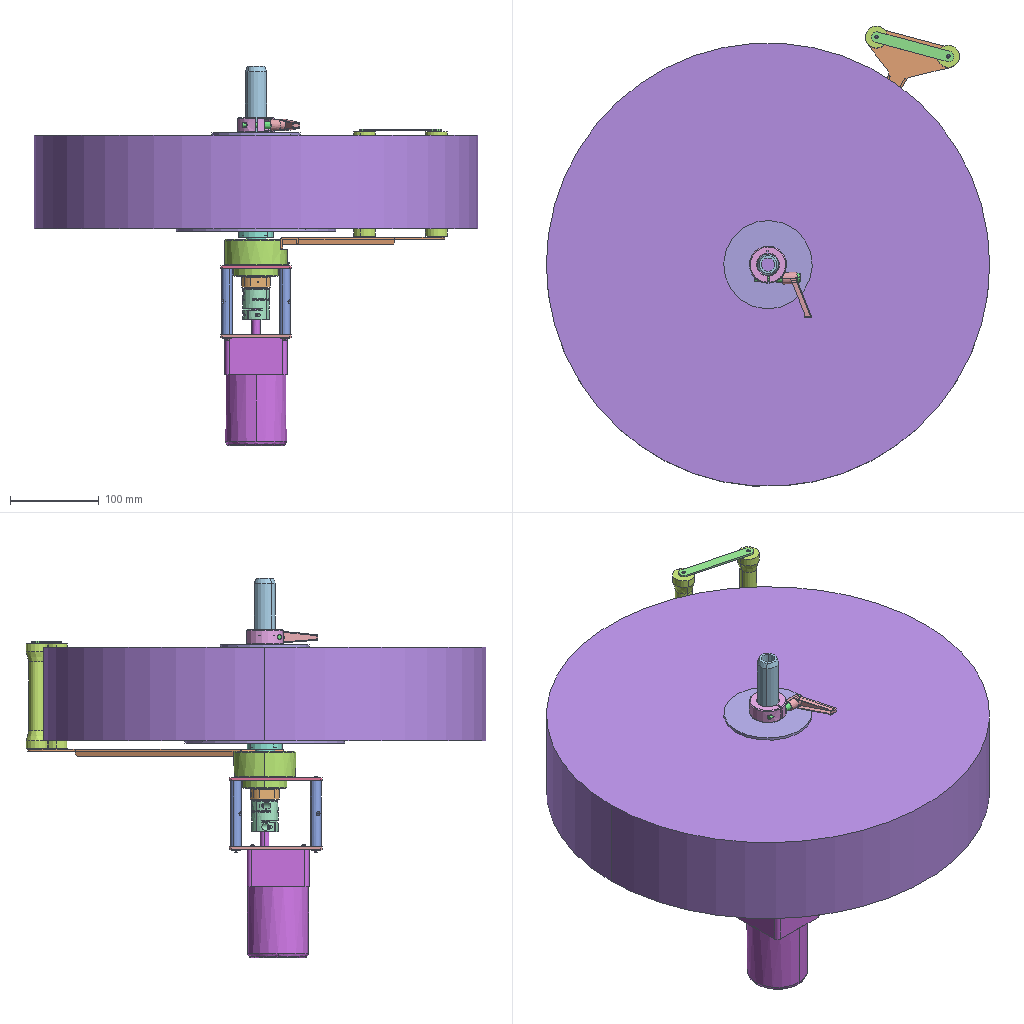Assembly | SolidWorks | 29 different items | 84 placed | box 500 x 519 x 428 mm
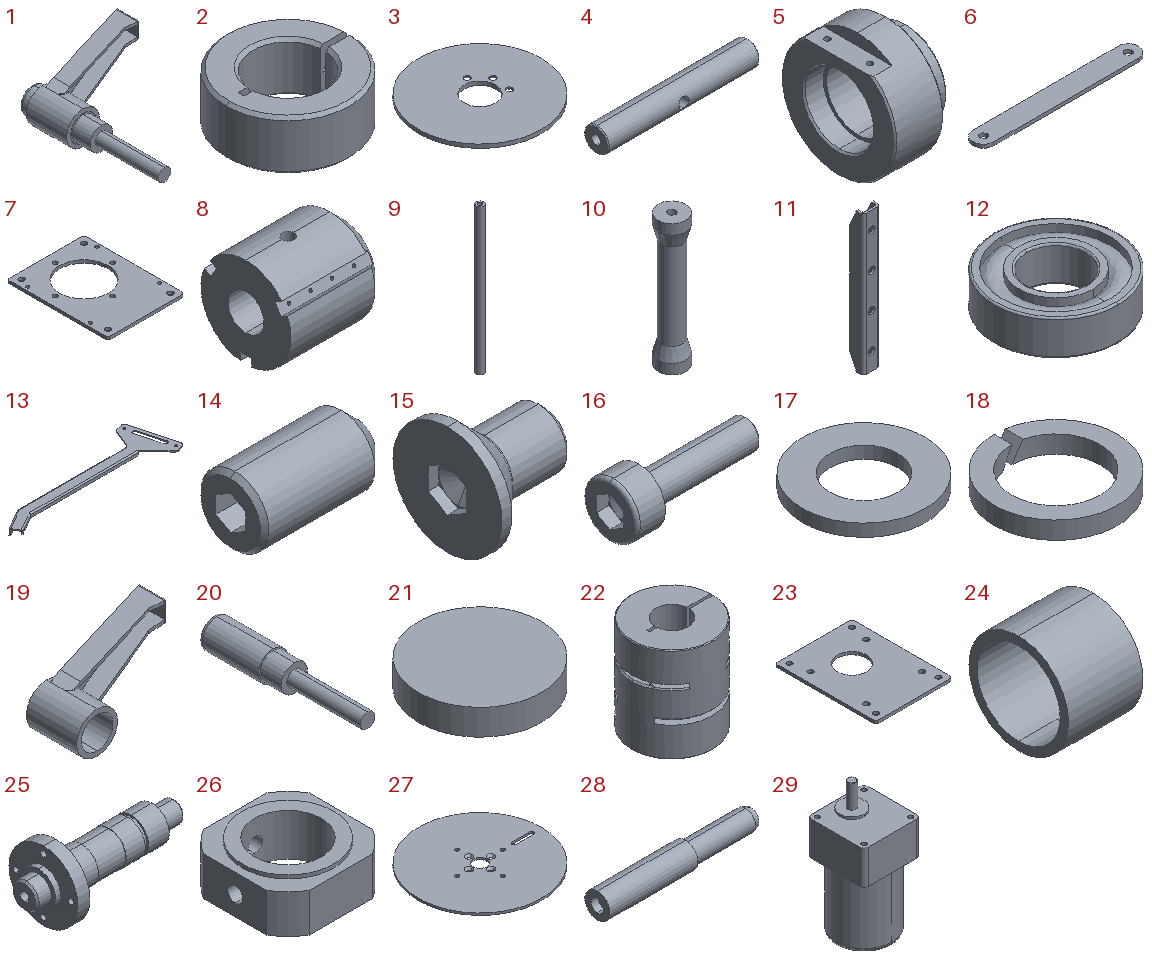Parts list (item | name | quantity | parent item | size | volume | features):
1 | (subassembly) | x1 | - | 51.5 x 63.5 x 13 mm | 4259 mm3 | -
2 | - | x1 | - | 41.976 x 42 x 17 mm | 13853 mm3 | features ICE 7, Chamfer 2, HoleWzd 2
3 | - | x1 | - | 100 x 100 x 3 mm | 21741 mm3 | features Extrusion 1, HoleWzd 1
4 | - | x4 | - | 75 x 12 x 12 mm | 7888 mm3 | features HoleWzd 2, Chamfer 1, Extrusion 1, ICE 1
5 | - | x1 | - | 42 x 70 x 70 mm | 81911 mm3 | features ICE 5, HoleWzd 2, Chamfer 1, CirPattern 1, Cut 1, Extrusion 1
6 | - | x1 | - | 96 x 12 x 2 mm | 2187 mm3 | features Extrusion 1, HoleWzd 1
7 | - | x1 | - | 80 x 105 x 3 mm | 18683 mm3 | features HoleWzd 2, Chamfer 1, Extrusion 1, ICE 1
8 | - | x1 | - | 80 x 75 x 74.698 mm | 269789 mm3 | features CirPattern 2, HoleWzd 2, ICE 2, Chamfer 1, Revolution 1
9 | - | x2 | - | 6 x 6 x 120 mm | 3214 mm3 | features HoleWzd 2, Extrusion 1
10 | - | x2 | - | 25 x 25 x 118 mm | 35489 mm3 | features Extrusion 1, RevCut 1
11 | - | x3 | - | 8.8 x 7 x 72 mm | 1341 mm3 | features Chamfer 2, FlatPattern 1, HoleWzd 1, SMBaseFlange 1, SheetMetal 1
12 | - | x2 | - | 42 x 42 x 12 mm | 10656 mm3 | features BaseBody 1
13 | - | x1 | - | 320.025 x 100.043 x 14 mm | 22575 mm3 | features ICE 5, Chamfer 2, HoleWzd 2, 3DProfileFeature 1, EdgeFlange 1, Fillet 1, FlatPattern 1, SMBaseFlange 1, SheetMetal 1
14 | - | x4 | - | 3 x 1.6 x 1.6 mm | 5.35 mm3 | features RevCut 2, Cut 1, LPattern 1, Revolution 1
15 | - | x4 | - | 10 x 11.34 x 11.34 mm | 423.495 mm3 | features RevCut 3, Chamfer 1, Cut 1, Fillet 1, LPattern 1, Revolution 1
16 | - | x20 | - | 7.6 x 3 x 3 mm | 21.652 mm3 | features Fillet 2, RevCut 2, Boss 1, Chamfer 1, Cut 1, Extrusion 1, LPattern 1
17 | - | x12 | - | 10 x 10 x 1 mm | 54.782 mm3 | features Extrusion 1
18 | - | x12 | - | 4.2 x 4.2 x 0.6 mm | 3.946 mm3 | features Cut 1, Extrusion 1
19 | - | x1 | in 1 | 51.5 x 31.3 x 13 mm | 1733 mm3 | features BaseBody 1, Shell 1
20 | - | x1 | in 1 | 10 x 52.5 x 10 mm | 2526 mm3 | features ICE 3, BaseBody 1
21 | - | x1 | - | 500 x 500 x 105 mm | 20616702 mm3 | features Extrusion 1
22 | - | x1 | - | 30 x 30 x 35 mm | 19054 mm3 | features BaseBody 1
23 | - | x1 | - | 80 x 105 x 3 mm | 22444 mm3 | features ICE 2, Chamfer 1, Extrusion 1, HoleWzd 1
24 | - | x1 | - | 18 x 24 x 24 mm | 2488 mm3 | features Extrusion 1
25 | - | x1 | - | 87 x 40 x 40 mm | 29288 mm3 | features HoleWzd 2, Chamfer 1, RevCut 1, Revolution 1
26 | - | x1 | - | 30 x 30 x 12 mm | 6216 mm3 | features HoleWzd 2, ICE 2, Extrusion 1
27 | - | x1 | - | 180 x 180 x 3 mm | 74053 mm3 | features Chamfer 1, Extrusion 1, ICE 1
28 | - | x1 | - | 183 x 30 x 30 mm | 80329 mm3 | features Chamfer 1, Revolution 1
29 | - | x1 | - | 70 x 70 x 154 mm | 503318 mm3 | features BaseBody 1
Mates (type | each side: item.copy, entity, surface, feature):
Coincident | 23.1 face plane Boss-Extrude1 | 4.1 face plane Boss-Extrude1
Concentric | 23.1 face cylinder Cut-Extrude1 | 4.1 face cylinder M5 Tapped Hole2
Coincident | 23.1 face plane Boss-Extrude1 | 4.2 face plane Boss-Extrude1
Concentric | 23.1 face cylinder Cut-Extrude1 | 4.2 face cylinder M5 Tapped Hole2
Coincident | 23.1 face plane Boss-Extrude1 | 4.3 face plane Boss-Extrude1
Concentric | 23.1 face cylinder Cut-Extrude1 | 4.3 face cylinder M5 Tapped Hole2
Coincident | 23.1 face plane Boss-Extrude1 | 4.4 face plane Boss-Extrude1
Concentric | 23.1 face cylinder Cut-Extrude1 | 4.4 face cylinder M5 Tapped Hole2
Coincident | 4.2 face plane Boss-Extrude1 | 7.1 face plane Boss-Extrude1
Concentric | 4.2 face cylinder M5 Tapped Hole1 | 7.1 face cylinder Cut-Extrude1
Concentric | 4.3 face cylinder M5 Tapped Hole1 | 7.1 face cylinder Cut-Extrude1
Concentric | 5.1 face cylinder Boss-Extrude1 | 7.1 face cylinder Cut-Extrude1
Concentric | 5.1 face cylinder Cut-Extrude1 | 25.1 face cylinder Revolve1
Concentric | 25.1 face cylinder Revolve1 | 27.1 face cylinder Boss-Extrude1
Concentric | 25.1 face cylinder M4 Tapped Hole1 | 27.1 face cylinder Cut-Extrude1
Coincident | 25.1 face plane Revolve1 | 27.1 face plane Boss-Extrude1
Concentric | 24.1 face cylinder Boss-Extrude1 | 25.1 face cylinder Revolve1
Coincident | 5.1 face plane Cut-Extrude3 | 24.1 face plane Boss-Extrude1
Concentric | 25.1 face cylinder Revolve1 | 26.1 face cylinder Cut-Extrude1
Coincident | 5.1 face plane Boss-Extrude3 | 26.1 face plane Boss-Extrude2
Concentric | 25.1 face cylinder Revolve1 | 28.1 face cylinder Revolve1
Coincident | 27.1 face plane Boss-Extrude1 | 28.1 face plane Revolve1
Concentric | 28.1 face cylinder Revolve1 | 8.1 face cylinder Revolve1
Coincident | 27.1 face plane Boss-Extrude1 | 8.1 face plane Revolve1
Concentric | 23.1 face cylinder Cut-Extrude1 | 29.1 face cylinder Import1
Coincident | 23.1 face plane Boss-Extrude1 | 29.1 face plane Import1
Concentric | 29.1 face cylinder Import1 | 23.1 face cylinder Cut-Extrude3
Concentric | 25.1 face cylinder Revolve1 | 22.1 face cylinder Import1
Concentric | 5.1 face cylinder Cut-Extrude3 | 12.1 face cylinder Import1
Coincident | 5.1 face plane Cut-Extrude3 | 12.1 face plane Import1
Concentric | 5.1 face cylinder Cut-Extrude1 | 12.2 face cylinder Import1
Coincident | 5.1 face plane Cut-Extrude1 | 12.2 face plane Import1
Concentric | 29.1 face cylinder Import1 | 17.1 face cylinder Base-Extrude
Coincident | 23.1 face plane Boss-Extrude1 | 17.1 face plane Base-Extrude
Concentric | 29.1 face cylinder Import1 | 17.2 face cylinder Base-Extrude
Coincident | 23.1 face plane Boss-Extrude1 | 17.2 face plane Base-Extrude
Concentric | 29.1 face cylinder Import1 | 17.3 face cylinder Base-Extrude
Coincident | 23.1 face plane Boss-Extrude1 | 17.3 face plane Base-Extrude
Concentric | 29.1 face cylinder Import1 | 17.4 face cylinder Base-Extrude
Coincident | 23.1 face plane Boss-Extrude1 | 17.4 face plane Base-Extrude
Concentric | 17.4 face cylinder Base-Extrude | 18.1 face cylinder Base-Extrude
Coincident | 17.4 face plane Base-Extrude | 18.1 face plane Base-Extrude
Concentric | 17.3 face cylinder Base-Extrude | 18.2 face cylinder Base-Extrude
Coincident | 17.3 face plane Base-Extrude | 18.2 face plane Base-Extrude
Concentric | 17.2 face cylinder Base-Extrude | 18.3 face cylinder Base-Extrude
Coincident | 17.2 face plane Base-Extrude | 18.3 face plane Base-Extrude
Concentric | 17.1 face cylinder Base-Extrude | 18.4 face cylinder Base-Extrude
Coincident | 17.1 face plane Base-Extrude | 18.4 face plane Base-Extrude
Concentric | 18.4 face cylinder Base-Extrude | 16.1 face cylinder BaseBody
Coincident | 18.4 face plane Base-Extrude | 16.1 face plane BaseHead
Concentric | 18.3 face cylinder Base-Extrude | 16.2 face cylinder BaseBody
Coincident | 18.3 face plane Base-Extrude | 16.2 face plane BaseHead
Concentric | 29.1 face cylinder Import1 | 16.3 face cylinder BaseBody
Coincident | 18.2 face plane Base-Extrude | 16.3 face plane BaseHead
Concentric | 18.1 face cylinder Base-Extrude | 16.4 face cylinder BaseBody
Coincident | 18.1 face plane Base-Extrude | 16.4 face plane BaseHead
Concentric | 23.1 face cylinder Cut-Extrude1 | 17.5 face cylinder Base-Extrude
Coincident | 23.1 face plane Boss-Extrude1 | 17.5 face plane Base-Extrude
Concentric | 23.1 face cylinder Cut-Extrude1 | 17.6 face cylinder Base-Extrude
Coincident | 23.1 face plane Boss-Extrude1 | 17.6 face plane Base-Extrude
Concentric | 23.1 face cylinder Cut-Extrude1 | 17.7 face cylinder Base-Extrude
Coincident | 23.1 face plane Boss-Extrude1 | 17.7 face plane Base-Extrude
Concentric | 23.1 face cylinder Cut-Extrude1 | 17.8 face cylinder Base-Extrude
Coincident | 23.1 face plane Boss-Extrude1 | 17.8 face plane Base-Extrude
Concentric | 17.8 face cylinder Base-Extrude | 18.5 face cylinder Base-Extrude
Coincident | 17.8 face plane Base-Extrude | 18.5 face plane Base-Extrude
Concentric | 17.7 face cylinder Base-Extrude | 18.6 face cylinder Base-Extrude
Coincident | 17.7 face plane Base-Extrude | 18.6 face plane Base-Extrude
Concentric | 17.5 face cylinder Base-Extrude | 18.7 face cylinder Base-Extrude
Coincident | 17.5 face plane Base-Extrude | 18.7 face plane Base-Extrude
Concentric | 17.6 face cylinder Base-Extrude | 18.8 face cylinder Base-Extrude
Coincident | 17.6 face plane Base-Extrude | 18.8 face plane Base-Extrude
Concentric | 18.8 face cylinder Base-Extrude | 16.5 face cylinder BaseBody
Coincident | 18.8 face plane Base-Extrude | 16.5 face plane BaseHead
Concentric | 18.7 face cylinder Base-Extrude | 16.6 face cylinder BaseBody
Coincident | 18.7 face plane Base-Extrude | 16.6 face plane BaseHead
Concentric | 18.6 face cylinder Base-Extrude | 16.7 face cylinder BaseBody
Coincident | 18.6 face plane Base-Extrude | 16.7 face plane BaseHead
Concentric | 18.5 face cylinder Base-Extrude | 16.8 face cylinder BaseBody
Coincident | 18.5 face plane Base-Extrude | 16.8 face plane BaseHead
Concentric | 22.1 face cylinder Import1 | 16.9 face cylinder BaseBody
Coincident | 22.1 face plane Import1 | 16.9 face plane BaseHead
Concentric | 22.1 face cylinder Import1 | 16.10 face cylinder BaseBody
Coincident | 22.1 face plane Import1 | 16.10 face plane BaseHead
Concentric | 26.1 face cylinder M5 Tapped Hole1 | 14.1 face cylinder Base
Tangent | 25.1 face cylinder Revolve1 | 14.1 face plane Base
Concentric | 26.1 face cylinder M5 Tapped Hole1 | 14.2 face cylinder Base
Tangent | 25.1 face cylinder Revolve1 | 14.2 face plane Base
Coincident | 5.1 face plane Boss-Extrude2 | 17.9 face plane Base-Extrude
Coincident | 5.1 face plane Boss-Extrude2 | 17.10 face plane Base-Extrude
Coincident | 5.1 face plane Boss-Extrude2 | 17.11 face plane Base-Extrude
Coincident | 5.1 face plane Boss-Extrude2 | 17.12 face plane Base-Extrude
Concentric | 17.12 face cylinder Base-Extrude | 18.9 face cylinder Base-Extrude
Coincident | 17.12 face plane Base-Extrude | 18.9 face plane Base-Extrude
Concentric | 17.11 face cylinder Base-Extrude | 18.10 face cylinder Base-Extrude
Coincident | 17.11 face plane Base-Extrude | 18.10 face plane Base-Extrude
Concentric | 17.10 face cylinder Base-Extrude | 18.11 face cylinder Base-Extrude
Coincident | 17.10 face plane Base-Extrude | 18.11 face plane Base-Extrude
Concentric | 17.9 face cylinder Base-Extrude | 18.12 face cylinder Base-Extrude
Coincident | 17.9 face plane Base-Extrude | 18.12 face plane Base-Extrude
Concentric | 18.11 face cylinder Base-Extrude | 16.11 face cylinder BaseBody
Coincident | 18.11 face plane Base-Extrude | 16.11 face plane BaseHead
Concentric | 18.10 face cylinder Base-Extrude | 16.12 face cylinder BaseBody
Coincident | 18.10 face plane Base-Extrude | 16.12 face plane BaseHead
Concentric | 18.12 face cylinder Base-Extrude | 16.13 face cylinder BaseBody
Coincident | 18.12 face plane Base-Extrude | 16.13 face plane BaseHead
Concentric | 18.9 face cylinder Base-Extrude | 16.14 face cylinder BaseBody
Coincident | 18.9 face plane Base-Extrude | 16.14 face plane BaseHead
Coincident | 27.1 face cone Chamfer1 | 15.1 face cone Base
Coincident | 27.1 face cone Chamfer1 | 15.2 face cone Base
Coincident | 27.1 face cone Chamfer1 | 15.3 face cone Base
Coincident | 27.1 face cone Chamfer1 | 15.4 face cone Base
Concentric | 28.1 face cylinder Revolve1 | 16.15 face cylinder BaseBody
Coincident | 28.1 face plane Revolve1 | 16.15 face plane BaseHead
Concentric | 7.1 face cylinder Cut-Extrude1 | 16.16 face cylinder BaseBody
Concentric | 7.1 face cylinder Cut-Extrude1 | 16.17 face cylinder BaseBody
Concentric | 7.1 face cylinder Cut-Extrude1 | 16.18 face cylinder BaseBody
Concentric | 8.1 face cylinder CirPattern1 | 14.3 face cylinder Base
Tangent | 28.1 face cylinder Revolve1 | 14.3 face plane Base
Concentric | 8.1 face cylinder M5 Tapped Hole1 | 14.4 face cylinder Base
Tangent | 28.1 face cylinder Revolve1 | 14.4 face plane Base
Concentric | 28.1 face cylinder Revolve1 | 2.1 face cylinder Boss-Extrude2
Coincident | 28.1 face plane Revolve1 | 3.1 face plane Boss-Extrude1
Concentric | 28.1 face cylinder Revolve1 | 3.1 face cylinder Boss-Extrude1
Coincident | 2.1 face plane Boss-Extrude2 | 3.1 face plane Boss-Extrude1
Concentric | 2.1 face cylinder M4 Tapped Hole1 | 3.1 face cylinder CSK for M4 Hex Socket Countersunk Cap Screw1
Concentric | 8.1 face cylinder Revolve1 | 21.1 face cylinder Boss-Extrude1
Coincident | 27.1 face plane Boss-Extrude1 | 21.1 face plane Boss-Extrude1
Coincident | 7.1 face plane Boss-Extrude1 | 16.16 face plane BaseHead
Coincident | 7.1 face plane Boss-Extrude1 | 16.18 face plane BaseHead
Coincident | 7.1 face plane Boss-Extrude1 | 16.17 face plane BaseHead
Coincident | 25.1 face plane Revolve1 | 12.2 face plane Import1
Coincident | 25.1 face plane Revolve1 | 22.1 face plane Import1
Concentric | 2.1 face cylinder Cut-Extrude3 | 20.1 face cylinder Import1
Coincident | 2.1 face plane Cut-Extrude4 | 20.1 face plane Boss-Extrude2
Coincident | 9.1 face plane Boss-Extrude1 | 6.1 face plane Boss-Extrude1
Concentric | 9.1 face cylinder Boss-Extrude1 | 6.1 face cylinder Ø4.2 (4.2) Diameter Hole1
Concentric | 9.2 face cylinder Boss-Extrude1 | 6.1 face cylinder Ø4.2 (4.2) Diameter Hole1
Concentric | 13.1 face cylinder Ø4.2 (4.2) Diameter Hole1 | 9.1 face cylinder Boss-Extrude1
Concentric | 13.1 face cylinder Ø4.2 (4.2) Diameter Hole1 | 9.2 face cylinder Boss-Extrude1
Coincident | 13.1 face plane Base-Flange1 | 9.2 face plane Boss-Extrude1
Coincident | 13.1 face plane Base-Flange1 | 9.1 face plane Boss-Extrude1
DistanceDim | 13.1 face plane Base-Flange1 | 10.1 face plane Boss-Extrude1
Concentric | 9.1 face cylinder Boss-Extrude1 | 10.1 face cylinder Boss-Extrude1
Concentric | 9.2 face cylinder Boss-Extrude1 | 10.2 face cylinder Boss-Extrude1
Coincident | 10.1 face plane Boss-Extrude1 | 10.2 face plane Boss-Extrude1
Coincident | 5.1 face plane Boss-Extrude2 | 7.1 face plane Boss-Extrude1
Coincident | 5.1 face plane Cut-Extrude4 | 13.1 face plane Edge-Flange4
Coincident | 5.1 face plane Cut-Extrude4 | 13.1 face plane Boss-Extrude3
Concentric | 7.1 face cylinder M4 Tapped Hole1 | 16.19 face cylinder BaseBody
DistanceDim | 16.19 face plane BaseHead | 7.1 face plane Boss-Extrude1
Concentric | 5.1 face cylinder M4 Tapped Hole3 | 13.1 face cylinder Ø4.5 (4.5) Diameter Hole2
Coincident | 8.1 face plane Cut-Extrude2 | 11.1 face plane Base-Flange1
Width | 11.1 face plane Base-Flange1 | 11.1 face plane Base-Flange1 | 8.1 face plane Cut-Extrude2 | 8.1 face plane Cut-Extrude2
Coincident | 27.1 face plane Boss-Extrude1 | 11.1 face plane Base-Flange1
Concentric | 5.1 face cylinder CirPattern1 | 7.1 face cylinder Ø4.5 (4.5) Diameter Hole1
Coincident | 11.1 face plane Base-Flange1 | 16.20 face plane BaseHead
Concentric | 8.1 face cylinder M3 Tapped Hole1 | 16.20 face cylinder BaseBody
Parallel | 7.1 face plane Boss-Extrude1 | 11.1 face plane Base-Flange1